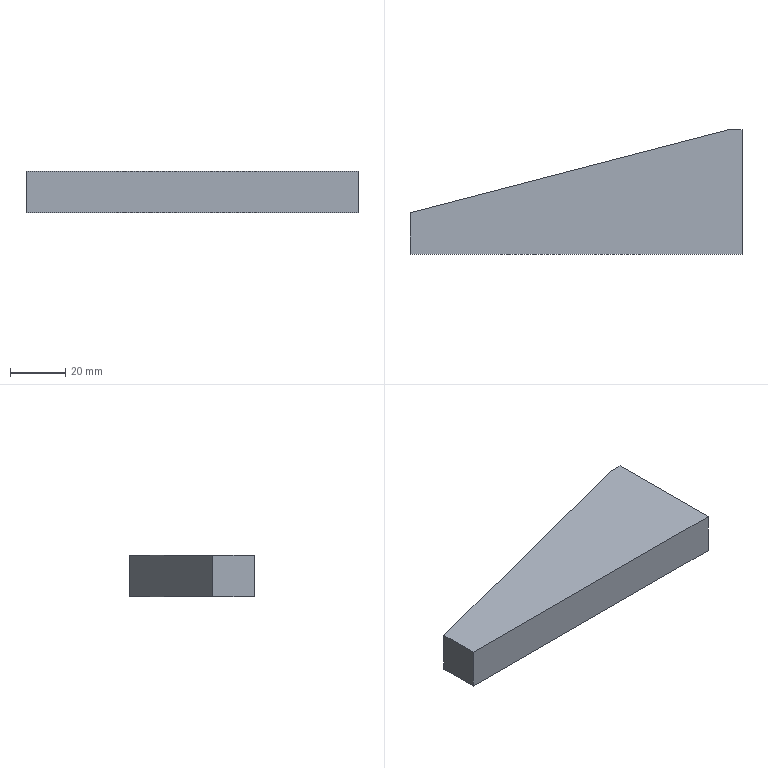Part | STEP file | 001-005-Shaft threading fixture reinforcing rib | 1 solid | 7 faces | box 120 x 45 x 15 mm | volume 55125 mm3 | plane 7
STEP:
#1=CARTESIAN_POINT('',(0.,0.,0.));
#2=DIRECTION('',(0.,0.,1.));
#3=DIRECTION('',(1.,0.,0.));
#4=AXIS2_PLACEMENT_3D('',#1,#2,#3);
#5=CARTESIAN_POINT('',(60.,-22.5,0.));
#6=VERTEX_POINT('',#5);
#7=CARTESIAN_POINT('',(60.,22.5,0.));
#8=VERTEX_POINT('',#7);
#9=CARTESIAN_POINT('',(60.,-22.5,0.));
#10=DIRECTION('',(0.,1.,0.));
#11=VECTOR('',#10,1.);
#12=LINE('',#9,#11);
#13=CARTESIAN_POINT('',(60.,-22.5,15.));
#14=DIRECTION('',(-1.,0.,0.));
#15=DIRECTION('',(0.,0.,1.));
#16=AXIS2_PLACEMENT_3D('',#13,#14,#15);
#17=PLANE('',#16);
#18=CARTESIAN_POINT('',(-15.,0.));
#19=DIRECTION('',(0.,1.));
#20=VECTOR('',#19,1.);
#21=LINE('',#18,#20);
#22=(GEOMETRIC_REPRESENTATION_CONTEXT(2)PARAMETRIC_REPRESENTATION_CONTEXT()REPRESENTATION_CONTEXT('',''));
#23=DEFINITIONAL_REPRESENTATION('',(#21),#22);
#24=PCURVE('',#17,#23);
#25=CARTESIAN_POINT('',(0.,0.,0.));
#26=DIRECTION('',(0.,0.,-1.));
#27=DIRECTION('',(-1.,0.,0.));
#28=AXIS2_PLACEMENT_3D('',#25,#26,#27);
#29=PLANE('',#28);
#30=CARTESIAN_POINT('',(-60.,-22.5));
#31=DIRECTION('',(0.,1.));
#32=VECTOR('',#31,1.);
#33=LINE('',#30,#32);
#34=(GEOMETRIC_REPRESENTATION_CONTEXT(2)PARAMETRIC_REPRESENTATION_CONTEXT()REPRESENTATION_CONTEXT('',''));
#35=DEFINITIONAL_REPRESENTATION('',(#33),#34);
#36=PCURVE('',#29,#35);
#37=SURFACE_CURVE('',#12,(#24,#36),.PCURVE_S1.);
#38=EDGE_CURVE('',#6,#8,#37,.T.);
#39=ORIENTED_EDGE('',*,*,#38,.T.);
#40=CARTESIAN_POINT('',(60.,22.5,15.));
#41=VERTEX_POINT('',#40);
#42=CARTESIAN_POINT('',(60.,22.5,15.));
#43=DIRECTION('',(0.,0.,-1.));
#44=VECTOR('',#43,1.);
#45=LINE('',#42,#44);
#46=CARTESIAN_POINT('',(0.,45.));
#47=DIRECTION('',(-1.,0.));
#48=VECTOR('',#47,1.);
#49=LINE('',#46,#48);
#50=(GEOMETRIC_REPRESENTATION_CONTEXT(2)PARAMETRIC_REPRESENTATION_CONTEXT()REPRESENTATION_CONTEXT('',''));
#51=DEFINITIONAL_REPRESENTATION('',(#49),#50);
#52=PCURVE('',#17,#51);
#53=CARTESIAN_POINT('',(-60.,22.5,15.));
#54=DIRECTION('',(0.,-1.,0.));
#55=DIRECTION('',(0.,0.,-1.));
#56=AXIS2_PLACEMENT_3D('',#53,#54,#55);
#57=PLANE('',#56);
#58=CARTESIAN_POINT('',(0.,120.));
#59=DIRECTION('',(1.,0.));
#60=VECTOR('',#59,1.);
#61=LINE('',#58,#60);
#62=(GEOMETRIC_REPRESENTATION_CONTEXT(2)PARAMETRIC_REPRESENTATION_CONTEXT()REPRESENTATION_CONTEXT('',''));
#63=DEFINITIONAL_REPRESENTATION('',(#61),#62);
#64=PCURVE('',#57,#63);
#65=SURFACE_CURVE('',#45,(#52,#64),.PCURVE_S1.);
#66=EDGE_CURVE('',#41,#8,#65,.T.);
#67=ORIENTED_EDGE('',*,*,#66,.F.);
#68=CARTESIAN_POINT('',(60.,-22.5,15.));
#69=VERTEX_POINT('',#68);
#70=CARTESIAN_POINT('',(60.,-22.5,15.));
#71=DIRECTION('',(0.,1.,0.));
#72=VECTOR('',#71,1.);
#73=LINE('',#70,#72);
#74=CARTESIAN_POINT('',(0.,0.));
#75=DIRECTION('',(0.,1.));
#76=VECTOR('',#75,1.);
#77=LINE('',#74,#76);
#78=(GEOMETRIC_REPRESENTATION_CONTEXT(2)PARAMETRIC_REPRESENTATION_CONTEXT()REPRESENTATION_CONTEXT('',''));
#79=DEFINITIONAL_REPRESENTATION('',(#77),#78);
#80=PCURVE('',#17,#79);
#81=CARTESIAN_POINT('',(0.,0.,15.));
#82=DIRECTION('',(0.,0.,-1.));
#83=DIRECTION('',(-1.,0.,0.));
#84=AXIS2_PLACEMENT_3D('',#81,#82,#83);
#85=PLANE('',#84);
#86=CARTESIAN_POINT('',(-60.,-22.5));
#87=DIRECTION('',(0.,1.));
#88=VECTOR('',#87,1.);
#89=LINE('',#86,#88);
#90=(GEOMETRIC_REPRESENTATION_CONTEXT(2)PARAMETRIC_REPRESENTATION_CONTEXT()REPRESENTATION_CONTEXT('',''));
#91=DEFINITIONAL_REPRESENTATION('',(#89),#90);
#92=PCURVE('',#85,#91);
#93=SURFACE_CURVE('',#73,(#80,#92),.PCURVE_S1.);
#94=EDGE_CURVE('',#69,#41,#93,.T.);
#95=ORIENTED_EDGE('',*,*,#94,.F.);
#96=CARTESIAN_POINT('',(60.,-22.5,15.));
#97=DIRECTION('',(0.,0.,-1.));
#98=VECTOR('',#97,1.);
#99=LINE('',#96,#98);
#100=CARTESIAN_POINT('',(0.,0.));
#101=DIRECTION('',(-1.,0.));
#102=VECTOR('',#101,1.);
#103=LINE('',#100,#102);
#104=(GEOMETRIC_REPRESENTATION_CONTEXT(2)PARAMETRIC_REPRESENTATION_CONTEXT()REPRESENTATION_CONTEXT('',''));
#105=DEFINITIONAL_REPRESENTATION('',(#103),#104);
#106=PCURVE('',#17,#105);
#107=CARTESIAN_POINT('',(-60.,-22.5,15.));
#108=DIRECTION('',(0.,1.,0.));
#109=DIRECTION('',(0.,0.,1.));
#110=AXIS2_PLACEMENT_3D('',#107,#108,#109);
#111=PLANE('',#110);
#112=CARTESIAN_POINT('',(0.,120.));
#113=DIRECTION('',(-1.,0.));
#114=VECTOR('',#113,1.);
#115=LINE('',#112,#114);
#116=(GEOMETRIC_REPRESENTATION_CONTEXT(2)PARAMETRIC_REPRESENTATION_CONTEXT()REPRESENTATION_CONTEXT('',''));
#117=DEFINITIONAL_REPRESENTATION('',(#115),#116);
#118=PCURVE('',#111,#117);
#119=SURFACE_CURVE('',#99,(#106,#118),.PCURVE_S1.);
#120=EDGE_CURVE('',#69,#6,#119,.T.);
#121=ORIENTED_EDGE('',*,*,#120,.T.);
#122=EDGE_LOOP('',(#39,#67,#95,#121));
#123=FACE_BOUND('',#122,.T.);
#124=ADVANCED_FACE('',(#123),#17,.F.);
#125=CARTESIAN_POINT('',(55.,22.5,0.));
#126=VERTEX_POINT('',#125);
#127=CARTESIAN_POINT('',(-60.,22.5,0.));
#128=DIRECTION('',(-1.,0.,0.));
#129=VECTOR('',#128,1.);
#130=LINE('',#127,#129);
#131=CARTESIAN_POINT('',(15.,0.));
#132=DIRECTION('',(0.,-1.));
#133=VECTOR('',#132,1.);
#134=LINE('',#131,#133);
#135=(GEOMETRIC_REPRESENTATION_CONTEXT(2)PARAMETRIC_REPRESENTATION_CONTEXT()REPRESENTATION_CONTEXT('',''));
#136=DEFINITIONAL_REPRESENTATION('',(#134),#135);
#137=PCURVE('',#57,#136);
#138=CARTESIAN_POINT('',(60.,22.5));
#139=DIRECTION('',(1.,0.));
#140=VECTOR('',#139,1.);
#141=LINE('',#138,#140);
#142=(GEOMETRIC_REPRESENTATION_CONTEXT(2)PARAMETRIC_REPRESENTATION_CONTEXT()REPRESENTATION_CONTEXT('',''));
#143=DEFINITIONAL_REPRESENTATION('',(#141),#142);
#144=PCURVE('',#29,#143);
#145=SURFACE_CURVE('',#130,(#137,#144),.PCURVE_S1.);
#146=EDGE_CURVE('',#8,#126,#145,.T.);
#147=ORIENTED_EDGE('',*,*,#146,.T.);
#148=CARTESIAN_POINT('',(55.,22.5,15.));
#149=VERTEX_POINT('',#148);
#150=CARTESIAN_POINT('',(55.,22.5,15.));
#151=DIRECTION('',(0.,0.,1.));
#152=VECTOR('',#151,1.);
#153=LINE('',#150,#152);
#154=CARTESIAN_POINT('',(0.,115.));
#155=DIRECTION('',(-1.,0.));
#156=VECTOR('',#155,1.);
#157=LINE('',#154,#156);
#158=(GEOMETRIC_REPRESENTATION_CONTEXT(2)PARAMETRIC_REPRESENTATION_CONTEXT()REPRESENTATION_CONTEXT('',''));
#159=DEFINITIONAL_REPRESENTATION('',(#157),#158);
#160=PCURVE('',#57,#159);
#161=CARTESIAN_POINT('',(-60.,-7.5,15.));
#162=DIRECTION('',(0.2524,-0.9676,0.));
#163=DIRECTION('',(0.,0.,-1.));
#164=AXIS2_PLACEMENT_3D('',#161,#162,#163);
#165=PLANE('',#164);
#166=CARTESIAN_POINT('',(0.,118.849));
#167=DIRECTION('',(-1.,0.));
#168=VECTOR('',#167,1.);
#169=LINE('',#166,#168);
#170=(GEOMETRIC_REPRESENTATION_CONTEXT(2)PARAMETRIC_REPRESENTATION_CONTEXT()REPRESENTATION_CONTEXT('',''));
#171=DEFINITIONAL_REPRESENTATION('',(#169),#170);
#172=PCURVE('',#165,#171);
#173=SURFACE_CURVE('',#153,(#160,#172),.PCURVE_S1.);
#174=EDGE_CURVE('',#126,#149,#173,.T.);
#175=ORIENTED_EDGE('',*,*,#174,.T.);
#176=CARTESIAN_POINT('',(-60.,22.5,15.));
#177=DIRECTION('',(-1.,0.,0.));
#178=VECTOR('',#177,1.);
#179=LINE('',#176,#178);
#180=CARTESIAN_POINT('',(0.,0.));
#181=DIRECTION('',(0.,-1.));
#182=VECTOR('',#181,1.);
#183=LINE('',#180,#182);
#184=(GEOMETRIC_REPRESENTATION_CONTEXT(2)PARAMETRIC_REPRESENTATION_CONTEXT()REPRESENTATION_CONTEXT('',''));
#185=DEFINITIONAL_REPRESENTATION('',(#183),#184);
#186=PCURVE('',#57,#185);
#187=CARTESIAN_POINT('',(60.,22.5));
#188=DIRECTION('',(1.,0.));
#189=VECTOR('',#188,1.);
#190=LINE('',#187,#189);
#191=(GEOMETRIC_REPRESENTATION_CONTEXT(2)PARAMETRIC_REPRESENTATION_CONTEXT()REPRESENTATION_CONTEXT('',''));
#192=DEFINITIONAL_REPRESENTATION('',(#190),#191);
#193=PCURVE('',#85,#192);
#194=SURFACE_CURVE('',#179,(#186,#193),.PCURVE_S1.);
#195=EDGE_CURVE('',#41,#149,#194,.T.);
#196=ORIENTED_EDGE('',*,*,#195,.F.);
#197=ORIENTED_EDGE('',*,*,#66,.T.);
#198=EDGE_LOOP('',(#147,#175,#196,#197));
#199=FACE_BOUND('',#198,.T.);
#200=ADVANCED_FACE('',(#199),#57,.F.);
#201=CARTESIAN_POINT('',(-60.,-7.5,15.));
#202=VERTEX_POINT('',#201);
#203=CARTESIAN_POINT('',(-60.,-22.5,15.));
#204=VERTEX_POINT('',#203);
#205=CARTESIAN_POINT('',(-60.,-22.5,15.));
#206=DIRECTION('',(0.,-1.,0.));
#207=VECTOR('',#206,1.);
#208=LINE('',#205,#207);
#209=CARTESIAN_POINT('',(-60.,-22.5,15.));
#210=DIRECTION('',(1.,0.,0.));
#211=DIRECTION('',(0.,0.,-1.));
#212=AXIS2_PLACEMENT_3D('',#209,#210,#211);
#213=PLANE('',#212);
#214=CARTESIAN_POINT('',(0.,0.));
#215=DIRECTION('',(0.,-1.));
#216=VECTOR('',#215,1.);
#217=LINE('',#214,#216);
#218=(GEOMETRIC_REPRESENTATION_CONTEXT(2)PARAMETRIC_REPRESENTATION_CONTEXT()REPRESENTATION_CONTEXT('',''));
#219=DEFINITIONAL_REPRESENTATION('',(#217),#218);
#220=PCURVE('',#213,#219);
#221=CARTESIAN_POINT('',(60.,-22.5));
#222=DIRECTION('',(0.,-1.));
#223=VECTOR('',#222,1.);
#224=LINE('',#221,#223);
#225=(GEOMETRIC_REPRESENTATION_CONTEXT(2)PARAMETRIC_REPRESENTATION_CONTEXT()REPRESENTATION_CONTEXT('',''));
#226=DEFINITIONAL_REPRESENTATION('',(#224),#225);
#227=PCURVE('',#85,#226);
#228=SURFACE_CURVE('',#208,(#220,#227),.PCURVE_S1.);
#229=EDGE_CURVE('',#202,#204,#228,.T.);
#230=ORIENTED_EDGE('',*,*,#229,.F.);
#231=CARTESIAN_POINT('',(-60.,-7.5,0.));
#232=VERTEX_POINT('',#231);
#233=CARTESIAN_POINT('',(-60.,-7.5,15.));
#234=DIRECTION('',(0.,0.,-1.));
#235=VECTOR('',#234,1.);
#236=LINE('',#233,#235);
#237=CARTESIAN_POINT('',(0.,15.));
#238=DIRECTION('',(1.,0.));
#239=VECTOR('',#238,1.);
#240=LINE('',#237,#239);
#241=(GEOMETRIC_REPRESENTATION_CONTEXT(2)PARAMETRIC_REPRESENTATION_CONTEXT()REPRESENTATION_CONTEXT('',''));
#242=DEFINITIONAL_REPRESENTATION('',(#240),#241);
#243=PCURVE('',#213,#242);
#244=CARTESIAN_POINT('',(0.,0.));
#245=DIRECTION('',(1.,0.));
#246=VECTOR('',#245,1.);
#247=LINE('',#244,#246);
#248=(GEOMETRIC_REPRESENTATION_CONTEXT(2)PARAMETRIC_REPRESENTATION_CONTEXT()REPRESENTATION_CONTEXT('',''));
#249=DEFINITIONAL_REPRESENTATION('',(#247),#248);
#250=PCURVE('',#165,#249);
#251=SURFACE_CURVE('',#236,(#243,#250),.PCURVE_S1.);
#252=EDGE_CURVE('',#202,#232,#251,.T.);
#253=ORIENTED_EDGE('',*,*,#252,.T.);
#254=CARTESIAN_POINT('',(-60.,-22.5,0.));
#255=VERTEX_POINT('',#254);
#256=CARTESIAN_POINT('',(-60.,-22.5,0.));
#257=DIRECTION('',(0.,-1.,0.));
#258=VECTOR('',#257,1.);
#259=LINE('',#256,#258);
#260=CARTESIAN_POINT('',(15.,0.));
#261=DIRECTION('',(0.,-1.));
#262=VECTOR('',#261,1.);
#263=LINE('',#260,#262);
#264=(GEOMETRIC_REPRESENTATION_CONTEXT(2)PARAMETRIC_REPRESENTATION_CONTEXT()REPRESENTATION_CONTEXT('',''));
#265=DEFINITIONAL_REPRESENTATION('',(#263),#264);
#266=PCURVE('',#213,#265);
#267=CARTESIAN_POINT('',(60.,-22.5));
#268=DIRECTION('',(0.,-1.));
#269=VECTOR('',#268,1.);
#270=LINE('',#267,#269);
#271=(GEOMETRIC_REPRESENTATION_CONTEXT(2)PARAMETRIC_REPRESENTATION_CONTEXT()REPRESENTATION_CONTEXT('',''));
#272=DEFINITIONAL_REPRESENTATION('',(#270),#271);
#273=PCURVE('',#29,#272);
#274=SURFACE_CURVE('',#259,(#266,#273),.PCURVE_S1.);
#275=EDGE_CURVE('',#232,#255,#274,.T.);
#276=ORIENTED_EDGE('',*,*,#275,.T.);
#277=CARTESIAN_POINT('',(-60.,-22.5,15.));
#278=DIRECTION('',(0.,0.,-1.));
#279=VECTOR('',#278,1.);
#280=LINE('',#277,#279);
#281=CARTESIAN_POINT('',(0.,0.));
#282=DIRECTION('',(1.,0.));
#283=VECTOR('',#282,1.);
#284=LINE('',#281,#283);
#285=(GEOMETRIC_REPRESENTATION_CONTEXT(2)PARAMETRIC_REPRESENTATION_CONTEXT()REPRESENTATION_CONTEXT('',''));
#286=DEFINITIONAL_REPRESENTATION('',(#284),#285);
#287=PCURVE('',#213,#286);
#288=CARTESIAN_POINT('',(0.,0.));
#289=DIRECTION('',(-1.,0.));
#290=VECTOR('',#289,1.);
#291=LINE('',#288,#290);
#292=(GEOMETRIC_REPRESENTATION_CONTEXT(2)PARAMETRIC_REPRESENTATION_CONTEXT()REPRESENTATION_CONTEXT('',''));
#293=DEFINITIONAL_REPRESENTATION('',(#291),#292);
#294=PCURVE('',#111,#293);
#295=SURFACE_CURVE('',#280,(#287,#294),.PCURVE_S1.);
#296=EDGE_CURVE('',#204,#255,#295,.T.);
#297=ORIENTED_EDGE('',*,*,#296,.F.);
#298=EDGE_LOOP('',(#230,#253,#276,#297));
#299=FACE_BOUND('',#298,.T.);
#300=ADVANCED_FACE('',(#299),#213,.F.);
#301=CARTESIAN_POINT('',(-60.,-22.5,0.));
#302=DIRECTION('',(1.,0.,0.));
#303=VECTOR('',#302,1.);
#304=LINE('',#301,#303);
#305=CARTESIAN_POINT('',(-15.,0.));
#306=DIRECTION('',(0.,1.));
#307=VECTOR('',#306,1.);
#308=LINE('',#305,#307);
#309=(GEOMETRIC_REPRESENTATION_CONTEXT(2)PARAMETRIC_REPRESENTATION_CONTEXT()REPRESENTATION_CONTEXT('',''));
#310=DEFINITIONAL_REPRESENTATION('',(#308),#309);
#311=PCURVE('',#111,#310);
#312=CARTESIAN_POINT('',(60.,-22.5));
#313=DIRECTION('',(-1.,0.));
#314=VECTOR('',#313,1.);
#315=LINE('',#312,#314);
#316=(GEOMETRIC_REPRESENTATION_CONTEXT(2)PARAMETRIC_REPRESENTATION_CONTEXT()REPRESENTATION_CONTEXT('',''));
#317=DEFINITIONAL_REPRESENTATION('',(#315),#316);
#318=PCURVE('',#29,#317);
#319=SURFACE_CURVE('',#304,(#311,#318),.PCURVE_S1.);
#320=EDGE_CURVE('',#255,#6,#319,.T.);
#321=ORIENTED_EDGE('',*,*,#320,.T.);
#322=ORIENTED_EDGE('',*,*,#120,.F.);
#323=CARTESIAN_POINT('',(-60.,-22.5,15.));
#324=DIRECTION('',(1.,0.,0.));
#325=VECTOR('',#324,1.);
#326=LINE('',#323,#325);
#327=CARTESIAN_POINT('',(0.,0.));
#328=DIRECTION('',(0.,1.));
#329=VECTOR('',#328,1.);
#330=LINE('',#327,#329);
#331=(GEOMETRIC_REPRESENTATION_CONTEXT(2)PARAMETRIC_REPRESENTATION_CONTEXT()REPRESENTATION_CONTEXT('',''));
#332=DEFINITIONAL_REPRESENTATION('',(#330),#331);
#333=PCURVE('',#111,#332);
#334=CARTESIAN_POINT('',(60.,-22.5));
#335=DIRECTION('',(-1.,0.));
#336=VECTOR('',#335,1.);
#337=LINE('',#334,#336);
#338=(GEOMETRIC_REPRESENTATION_CONTEXT(2)PARAMETRIC_REPRESENTATION_CONTEXT()REPRESENTATION_CONTEXT('',''));
#339=DEFINITIONAL_REPRESENTATION('',(#337),#338);
#340=PCURVE('',#85,#339);
#341=SURFACE_CURVE('',#326,(#333,#340),.PCURVE_S1.);
#342=EDGE_CURVE('',#204,#69,#341,.T.);
#343=ORIENTED_EDGE('',*,*,#342,.F.);
#344=ORIENTED_EDGE('',*,*,#296,.T.);
#345=EDGE_LOOP('',(#321,#322,#343,#344));
#346=FACE_BOUND('',#345,.T.);
#347=ADVANCED_FACE('',(#346),#111,.F.);
#348=ORIENTED_EDGE('',*,*,#195,.T.);
#349=CARTESIAN_POINT('',(-60.,-7.5,15.));
#350=DIRECTION('',(-0.9676,-0.2524,0.));
#351=VECTOR('',#350,1.);
#352=LINE('',#349,#351);
#353=CARTESIAN_POINT('',(60.,-7.5));
#354=DIRECTION('',(0.9676,-0.2524));
#355=VECTOR('',#354,1.);
#356=LINE('',#353,#355);
#357=(GEOMETRIC_REPRESENTATION_CONTEXT(2)PARAMETRIC_REPRESENTATION_CONTEXT()REPRESENTATION_CONTEXT('',''));
#358=DEFINITIONAL_REPRESENTATION('',(#356),#357);
#359=PCURVE('',#85,#358);
#360=CARTESIAN_POINT('',(0.,0.));
#361=DIRECTION('',(0.,-1.));
#362=VECTOR('',#361,1.);
#363=LINE('',#360,#362);
#364=(GEOMETRIC_REPRESENTATION_CONTEXT(2)PARAMETRIC_REPRESENTATION_CONTEXT()REPRESENTATION_CONTEXT('',''));
#365=DEFINITIONAL_REPRESENTATION('',(#363),#364);
#366=PCURVE('',#165,#365);
#367=SURFACE_CURVE('',#352,(#359,#366),.PCURVE_S1.);
#368=EDGE_CURVE('',#149,#202,#367,.T.);
#369=ORIENTED_EDGE('',*,*,#368,.T.);
#370=ORIENTED_EDGE('',*,*,#229,.T.);
#371=ORIENTED_EDGE('',*,*,#342,.T.);
#372=ORIENTED_EDGE('',*,*,#94,.T.);
#373=EDGE_LOOP('',(#348,#369,#370,#371,#372));
#374=FACE_BOUND('',#373,.T.);
#375=ADVANCED_FACE('',(#374),#85,.F.);
#376=ORIENTED_EDGE('',*,*,#275,.F.);
#377=CARTESIAN_POINT('',(-1.991,7.633,0.));
#378=DIRECTION('',(0.9676,0.2524,0.));
#379=VECTOR('',#378,1.);
#380=LINE('',#377,#379);
#381=CARTESIAN_POINT('',(1.991,7.633));
#382=DIRECTION('',(-0.9676,0.2524));
#383=VECTOR('',#382,1.);
#384=LINE('',#381,#383);
#385=(GEOMETRIC_REPRESENTATION_CONTEXT(2)PARAMETRIC_REPRESENTATION_CONTEXT()REPRESENTATION_CONTEXT('',''));
#386=DEFINITIONAL_REPRESENTATION('',(#384),#385);
#387=PCURVE('',#29,#386);
#388=CARTESIAN_POINT('',(15.,59.95));
#389=DIRECTION('',(0.,1.));
#390=VECTOR('',#389,1.);
#391=LINE('',#388,#390);
#392=(GEOMETRIC_REPRESENTATION_CONTEXT(2)PARAMETRIC_REPRESENTATION_CONTEXT()REPRESENTATION_CONTEXT('',''));
#393=DEFINITIONAL_REPRESENTATION('',(#391),#392);
#394=PCURVE('',#165,#393);
#395=SURFACE_CURVE('',#380,(#387,#394),.PCURVE_S1.);
#396=EDGE_CURVE('',#232,#126,#395,.T.);
#397=ORIENTED_EDGE('',*,*,#396,.T.);
#398=ORIENTED_EDGE('',*,*,#146,.F.);
#399=ORIENTED_EDGE('',*,*,#38,.F.);
#400=ORIENTED_EDGE('',*,*,#320,.F.);
#401=EDGE_LOOP('',(#376,#397,#398,#399,#400));
#402=FACE_BOUND('',#401,.T.);
#403=ADVANCED_FACE('',(#402),#29,.T.);
#404=ORIENTED_EDGE('',*,*,#368,.F.);
#405=ORIENTED_EDGE('',*,*,#174,.F.);
#406=ORIENTED_EDGE('',*,*,#396,.F.);
#407=ORIENTED_EDGE('',*,*,#252,.F.);
#408=EDGE_LOOP('',(#404,#405,#406,#407));
#409=FACE_BOUND('',#408,.T.);
#410=ADVANCED_FACE('',(#409),#165,.F.);
#411=CLOSED_SHELL('',(#124,#200,#300,#347,#375,#403,#410));
#412=MANIFOLD_SOLID_BREP('',#411);
#413=(LENGTH_UNIT()NAMED_UNIT(*)SI_UNIT(.MILLI.,.METRE.));
#414=UNCERTAINTY_MEASURE_WITH_UNIT(LENGTH_MEASURE(0.0000001),#413,'','');
#415=(NAMED_UNIT(*)PLANE_ANGLE_UNIT()SI_UNIT($,.RADIAN.));
#416=(NAMED_UNIT(*)SI_UNIT($,.STERADIAN.)SOLID_ANGLE_UNIT());
#417=(GEOMETRIC_REPRESENTATION_CONTEXT(3)GLOBAL_UNCERTAINTY_ASSIGNED_CONTEXT((#414))GLOBAL_UNIT_ASSIGNED_CONTEXT((#413,#415,#416))REPRESENTATION_CONTEXT('',''));
#418=ADVANCED_BREP_SHAPE_REPRESENTATION('',(#4,#412),#417);